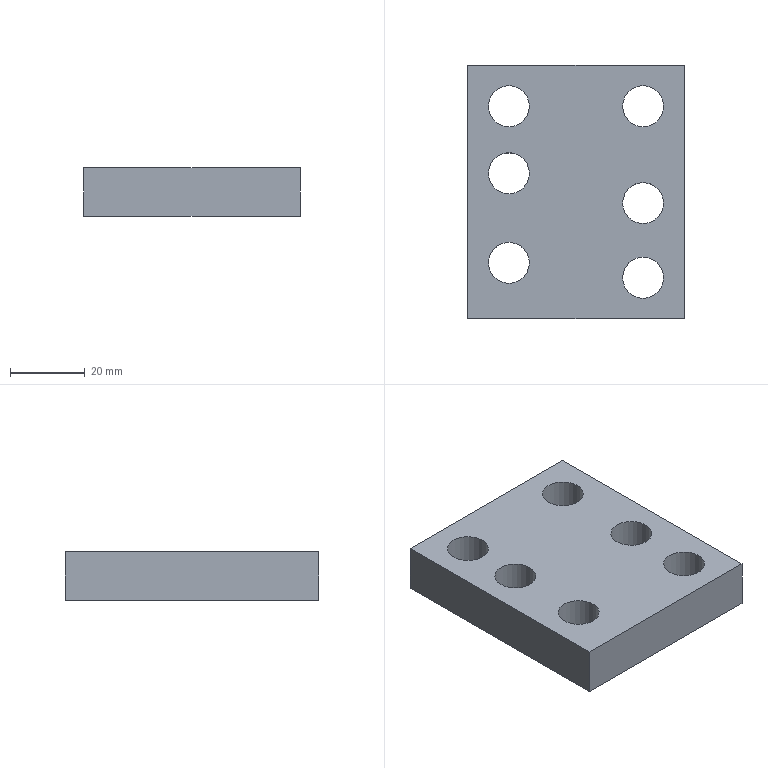Part | NX | features solid 2 | 1 solid | 12 faces | box 58 x 68 x 13 mm | volume 43859 mm3 | plane 6 | cylinder 6 | commonest cylinder face diameters 11 x6
STEP:
#1=CARTESIAN_POINT('',(1257.079,107.904,53.));
#2=VERTEX_POINT('',#1);
#3=CARTESIAN_POINT('',(1257.079,107.904,40.));
#4=VERTEX_POINT('',#3);
#5=CARTESIAN_POINT('',(1257.079,107.904,40.));
#6=DIRECTION('',(0.,0.,1.));
#7=VECTOR('',#6,1000.);
#8=LINE('',#5,#7);
#9=EDGE_CURVE('',#2,#4,#8,.F.);
#10=ORIENTED_EDGE('',*,*,#9,.T.);
#11=CARTESIAN_POINT('',(1315.079,107.904,40.));
#12=VERTEX_POINT('',#11);
#13=CARTESIAN_POINT('',(1286.079,107.904,40.));
#14=DIRECTION('',(1.,0.,0.));
#15=VECTOR('',#14,1000.);
#16=LINE('',#13,#15);
#17=EDGE_CURVE('',#12,#4,#16,.F.);
#18=ORIENTED_EDGE('',*,*,#17,.F.);
#19=CARTESIAN_POINT('',(1315.079,107.904,53.));
#20=VERTEX_POINT('',#19);
#21=CARTESIAN_POINT('',(1315.079,107.904,40.));
#22=DIRECTION('',(0.,0.,1.));
#23=VECTOR('',#22,1000.);
#24=LINE('',#21,#23);
#25=EDGE_CURVE('',#20,#12,#24,.F.);
#26=ORIENTED_EDGE('',*,*,#25,.F.);
#27=CARTESIAN_POINT('',(2087.158,107.904,53.));
#28=DIRECTION('',(1.,0.,0.));
#29=VECTOR('',#28,1000.);
#30=LINE('',#27,#29);
#31=EDGE_CURVE('',#20,#2,#30,.F.);
#32=ORIENTED_EDGE('',*,*,#31,.T.);
#33=EDGE_LOOP('',(#10,#18,#26,#32));
#34=FACE_BOUND('',#33,.T.);
#35=CARTESIAN_POINT('',(1286.079,107.904,40.));
#36=DIRECTION('',(0.,1.,0.));
#37=DIRECTION('',(1.,0.,0.));
#38=AXIS2_PLACEMENT_3D('',#35,#36,#37);
#39=PLANE('',#38);
#40=ADVANCED_FACE('',(#34),#39,.F.);
#41=ORIENTED_EDGE('',*,*,#25,.T.);
#42=CARTESIAN_POINT('',(1315.079,175.904,40.));
#43=VERTEX_POINT('',#42);
#44=CARTESIAN_POINT('',(1315.079,141.904,40.));
#45=DIRECTION('',(0.,1.,0.));
#46=VECTOR('',#45,1000.);
#47=LINE('',#44,#46);
#48=EDGE_CURVE('',#43,#12,#47,.F.);
#49=ORIENTED_EDGE('',*,*,#48,.F.);
#50=CARTESIAN_POINT('',(1315.079,175.904,53.));
#51=VERTEX_POINT('',#50);
#52=CARTESIAN_POINT('',(1315.079,175.904,40.));
#53=DIRECTION('',(0.,0.,1.));
#54=VECTOR('',#53,1000.);
#55=LINE('',#52,#54);
#56=EDGE_CURVE('',#51,#43,#55,.F.);
#57=ORIENTED_EDGE('',*,*,#56,.F.);
#58=CARTESIAN_POINT('',(1315.079,0.000000688,53.));
#59=DIRECTION('',(0.,1.,0.));
#60=VECTOR('',#59,1000.);
#61=LINE('',#58,#60);
#62=EDGE_CURVE('',#51,#20,#61,.F.);
#63=ORIENTED_EDGE('',*,*,#62,.T.);
#64=EDGE_LOOP('',(#41,#49,#57,#63));
#65=FACE_BOUND('',#64,.T.);
#66=CARTESIAN_POINT('',(1315.079,141.904,40.));
#67=DIRECTION('',(-1.,0.,0.));
#68=DIRECTION('',(0.,1.,0.));
#69=AXIS2_PLACEMENT_3D('',#66,#67,#68);
#70=PLANE('',#69);
#71=ADVANCED_FACE('',(#65),#70,.F.);
#72=ORIENTED_EDGE('',*,*,#56,.T.);
#73=CARTESIAN_POINT('',(1257.079,175.904,40.));
#74=VERTEX_POINT('',#73);
#75=CARTESIAN_POINT('',(1286.079,175.904,40.));
#76=DIRECTION('',(-1.,0.,0.));
#77=VECTOR('',#76,1000.);
#78=LINE('',#75,#77);
#79=EDGE_CURVE('',#74,#43,#78,.F.);
#80=ORIENTED_EDGE('',*,*,#79,.F.);
#81=CARTESIAN_POINT('',(1257.079,175.904,53.));
#82=VERTEX_POINT('',#81);
#83=CARTESIAN_POINT('',(1257.079,175.904,40.));
#84=DIRECTION('',(0.,0.,1.));
#85=VECTOR('',#84,1000.);
#86=LINE('',#83,#85);
#87=EDGE_CURVE('',#82,#74,#86,.F.);
#88=ORIENTED_EDGE('',*,*,#87,.F.);
#89=CARTESIAN_POINT('',(2087.158,175.904,53.));
#90=DIRECTION('',(-1.,0.,0.));
#91=VECTOR('',#90,1000.);
#92=LINE('',#89,#91);
#93=EDGE_CURVE('',#82,#51,#92,.F.);
#94=ORIENTED_EDGE('',*,*,#93,.T.);
#95=EDGE_LOOP('',(#72,#80,#88,#94));
#96=FACE_BOUND('',#95,.T.);
#97=CARTESIAN_POINT('',(1286.079,175.904,40.));
#98=DIRECTION('',(0.,-1.,0.));
#99=DIRECTION('',(-1.,0.,0.));
#100=AXIS2_PLACEMENT_3D('',#97,#98,#99);
#101=PLANE('',#100);
#102=ADVANCED_FACE('',(#96),#101,.F.);
#103=CARTESIAN_POINT('',(1273.579,146.904,40.));
#104=VERTEX_POINT('',#103);
#105=CARTESIAN_POINT('',(1268.079,146.904,40.));
#106=DIRECTION('',(0.,0.,-1.));
#107=DIRECTION('',(1.,0.,0.));
#108=AXIS2_PLACEMENT_3D('',#105,#106,#107);
#109=CIRCLE('',#108,5.5);
#110=EDGE_CURVE('',#104,#104,#109,.T.);
#111=ORIENTED_EDGE('',*,*,#110,.T.);
#112=EDGE_LOOP('',(#111));
#113=FACE_BOUND('',#112,.T.);
#114=CARTESIAN_POINT('',(1262.579,146.904,53.));
#115=VERTEX_POINT('',#114);
#116=CARTESIAN_POINT('',(1268.079,146.904,53.));
#117=DIRECTION('',(0.,0.,-1.));
#118=DIRECTION('',(-1.,0.,0.));
#119=AXIS2_PLACEMENT_3D('',#116,#117,#118);
#120=CIRCLE('',#119,5.5);
#121=EDGE_CURVE('',#115,#115,#120,.T.);
#122=ORIENTED_EDGE('',*,*,#121,.F.);
#123=EDGE_LOOP('',(#122));
#124=FACE_BOUND('',#123,.T.);
#125=CARTESIAN_POINT('',(1268.079,146.904,40.));
#126=DIRECTION('',(0.,0.,-1.));
#127=DIRECTION('',(1.,0.,0.));
#128=AXIS2_PLACEMENT_3D('',#125,#126,#127);
#129=CYLINDRICAL_SURFACE('',#128,5.5);
#130=ADVANCED_FACE('',(#113,#124),#129,.F.);
#131=CARTESIAN_POINT('',(1309.579,138.904,40.));
#132=VERTEX_POINT('',#131);
#133=CARTESIAN_POINT('',(1304.079,138.904,40.));
#134=DIRECTION('',(0.,0.,-1.));
#135=DIRECTION('',(1.,0.,0.));
#136=AXIS2_PLACEMENT_3D('',#133,#134,#135);
#137=CIRCLE('',#136,5.5);
#138=EDGE_CURVE('',#132,#132,#137,.F.);
#139=ORIENTED_EDGE('',*,*,#138,.F.);
#140=EDGE_LOOP('',(#139));
#141=FACE_BOUND('',#140,.T.);
#142=CARTESIAN_POINT('',(1298.579,138.904,53.));
#143=VERTEX_POINT('',#142);
#144=CARTESIAN_POINT('',(1304.079,138.904,53.));
#145=DIRECTION('',(0.,0.,-1.));
#146=DIRECTION('',(-1.,0.,0.));
#147=AXIS2_PLACEMENT_3D('',#144,#145,#146);
#148=CIRCLE('',#147,5.5);
#149=EDGE_CURVE('',#143,#143,#148,.F.);
#150=ORIENTED_EDGE('',*,*,#149,.T.);
#151=EDGE_LOOP('',(#150));
#152=FACE_BOUND('',#151,.T.);
#153=CARTESIAN_POINT('',(1304.079,138.904,40.));
#154=DIRECTION('',(0.,0.,-1.));
#155=DIRECTION('',(1.,0.,0.));
#156=AXIS2_PLACEMENT_3D('',#153,#154,#155);
#157=CYLINDRICAL_SURFACE('',#156,5.5);
#158=ADVANCED_FACE('',(#141,#152),#157,.F.);
#159=CARTESIAN_POINT('',(1273.579,122.904,40.));
#160=VERTEX_POINT('',#159);
#161=CARTESIAN_POINT('',(1268.079,122.904,40.));
#162=DIRECTION('',(0.,0.,-1.));
#163=DIRECTION('',(1.,0.,0.));
#164=AXIS2_PLACEMENT_3D('',#161,#162,#163);
#165=CIRCLE('',#164,5.5);
#166=EDGE_CURVE('',#160,#160,#165,.T.);
#167=ORIENTED_EDGE('',*,*,#166,.T.);
#168=EDGE_LOOP('',(#167));
#169=FACE_BOUND('',#168,.T.);
#170=CARTESIAN_POINT('',(1262.579,122.904,53.));
#171=VERTEX_POINT('',#170);
#172=CARTESIAN_POINT('',(1268.079,122.904,53.));
#173=DIRECTION('',(0.,0.,-1.));
#174=DIRECTION('',(-1.,0.,0.));
#175=AXIS2_PLACEMENT_3D('',#172,#173,#174);
#176=CIRCLE('',#175,5.5);
#177=EDGE_CURVE('',#171,#171,#176,.T.);
#178=ORIENTED_EDGE('',*,*,#177,.F.);
#179=EDGE_LOOP('',(#178));
#180=FACE_BOUND('',#179,.T.);
#181=CARTESIAN_POINT('',(1268.079,122.904,40.));
#182=DIRECTION('',(0.,0.,-1.));
#183=DIRECTION('',(1.,0.,0.));
#184=AXIS2_PLACEMENT_3D('',#181,#182,#183);
#185=CYLINDRICAL_SURFACE('',#184,5.5);
#186=ADVANCED_FACE('',(#169,#180),#185,.F.);
#187=CARTESIAN_POINT('',(1273.579,164.904,40.));
#188=VERTEX_POINT('',#187);
#189=CARTESIAN_POINT('',(1268.079,164.904,40.));
#190=DIRECTION('',(0.,0.,-1.));
#191=DIRECTION('',(1.,0.,0.));
#192=AXIS2_PLACEMENT_3D('',#189,#190,#191);
#193=CIRCLE('',#192,5.5);
#194=EDGE_CURVE('',#188,#188,#193,.T.);
#195=ORIENTED_EDGE('',*,*,#194,.T.);
#196=EDGE_LOOP('',(#195));
#197=FACE_BOUND('',#196,.T.);
#198=CARTESIAN_POINT('',(1262.579,164.904,53.));
#199=VERTEX_POINT('',#198);
#200=CARTESIAN_POINT('',(1268.079,164.904,53.));
#201=DIRECTION('',(0.,0.,-1.));
#202=DIRECTION('',(-1.,0.,0.));
#203=AXIS2_PLACEMENT_3D('',#200,#201,#202);
#204=CIRCLE('',#203,5.5);
#205=EDGE_CURVE('',#199,#199,#204,.T.);
#206=ORIENTED_EDGE('',*,*,#205,.F.);
#207=EDGE_LOOP('',(#206));
#208=FACE_BOUND('',#207,.T.);
#209=CARTESIAN_POINT('',(1268.079,164.904,40.));
#210=DIRECTION('',(0.,0.,-1.));
#211=DIRECTION('',(1.,0.,0.));
#212=AXIS2_PLACEMENT_3D('',#209,#210,#211);
#213=CYLINDRICAL_SURFACE('',#212,5.5);
#214=ADVANCED_FACE('',(#197,#208),#213,.F.);
#215=CARTESIAN_POINT('',(1309.579,164.904,40.));
#216=VERTEX_POINT('',#215);
#217=CARTESIAN_POINT('',(1304.079,164.904,40.));
#218=DIRECTION('',(0.,0.,-1.));
#219=DIRECTION('',(1.,0.,0.));
#220=AXIS2_PLACEMENT_3D('',#217,#218,#219);
#221=CIRCLE('',#220,5.5);
#222=EDGE_CURVE('',#216,#216,#221,.T.);
#223=ORIENTED_EDGE('',*,*,#222,.T.);
#224=EDGE_LOOP('',(#223));
#225=FACE_BOUND('',#224,.T.);
#226=CARTESIAN_POINT('',(1298.579,164.904,53.));
#227=VERTEX_POINT('',#226);
#228=CARTESIAN_POINT('',(1304.079,164.904,53.));
#229=DIRECTION('',(0.,0.,-1.));
#230=DIRECTION('',(-1.,0.,0.));
#231=AXIS2_PLACEMENT_3D('',#228,#229,#230);
#232=CIRCLE('',#231,5.5);
#233=EDGE_CURVE('',#227,#227,#232,.T.);
#234=ORIENTED_EDGE('',*,*,#233,.F.);
#235=EDGE_LOOP('',(#234));
#236=FACE_BOUND('',#235,.T.);
#237=CARTESIAN_POINT('',(1304.079,164.904,40.));
#238=DIRECTION('',(0.,0.,-1.));
#239=DIRECTION('',(1.,0.,0.));
#240=AXIS2_PLACEMENT_3D('',#237,#238,#239);
#241=CYLINDRICAL_SURFACE('',#240,5.5);
#242=ADVANCED_FACE('',(#225,#236),#241,.F.);
#243=CARTESIAN_POINT('',(1309.579,118.904,40.));
#244=VERTEX_POINT('',#243);
#245=CARTESIAN_POINT('',(1304.079,118.904,40.));
#246=DIRECTION('',(0.,0.,-1.));
#247=DIRECTION('',(1.,0.,0.));
#248=AXIS2_PLACEMENT_3D('',#245,#246,#247);
#249=CIRCLE('',#248,5.5);
#250=EDGE_CURVE('',#244,#244,#249,.F.);
#251=ORIENTED_EDGE('',*,*,#250,.F.);
#252=EDGE_LOOP('',(#251));
#253=FACE_BOUND('',#252,.T.);
#254=CARTESIAN_POINT('',(1298.579,118.904,53.));
#255=VERTEX_POINT('',#254);
#256=CARTESIAN_POINT('',(1304.079,118.904,53.));
#257=DIRECTION('',(0.,0.,-1.));
#258=DIRECTION('',(-1.,0.,0.));
#259=AXIS2_PLACEMENT_3D('',#256,#257,#258);
#260=CIRCLE('',#259,5.5);
#261=EDGE_CURVE('',#255,#255,#260,.F.);
#262=ORIENTED_EDGE('',*,*,#261,.T.);
#263=EDGE_LOOP('',(#262));
#264=FACE_BOUND('',#263,.T.);
#265=CARTESIAN_POINT('',(1304.079,118.904,40.));
#266=DIRECTION('',(0.,0.,-1.));
#267=DIRECTION('',(1.,0.,0.));
#268=AXIS2_PLACEMENT_3D('',#265,#266,#267);
#269=CYLINDRICAL_SURFACE('',#268,5.5);
#270=ADVANCED_FACE('',(#253,#264),#269,.F.);
#271=CARTESIAN_POINT('',(1257.079,0.000000688,53.));
#272=DIRECTION('',(0.,-1.,0.));
#273=VECTOR('',#272,1000.);
#274=LINE('',#271,#273);
#275=EDGE_CURVE('',#2,#82,#274,.F.);
#276=ORIENTED_EDGE('',*,*,#275,.T.);
#277=ORIENTED_EDGE('',*,*,#87,.T.);
#278=CARTESIAN_POINT('',(1257.079,141.904,40.));
#279=DIRECTION('',(0.,-1.,0.));
#280=VECTOR('',#279,1000.);
#281=LINE('',#278,#280);
#282=EDGE_CURVE('',#4,#74,#281,.F.);
#283=ORIENTED_EDGE('',*,*,#282,.F.);
#284=ORIENTED_EDGE('',*,*,#9,.F.);
#285=EDGE_LOOP('',(#276,#277,#283,#284));
#286=FACE_BOUND('',#285,.T.);
#287=CARTESIAN_POINT('',(1257.079,141.904,40.));
#288=DIRECTION('',(1.,0.,0.));
#289=DIRECTION('',(0.,-1.,0.));
#290=AXIS2_PLACEMENT_3D('',#287,#288,#289);
#291=PLANE('',#290);
#292=ADVANCED_FACE('',(#286),#291,.F.);
#293=ORIENTED_EDGE('',*,*,#110,.F.);
#294=EDGE_LOOP('',(#293));
#295=FACE_BOUND('',#294,.T.);
#296=ORIENTED_EDGE('',*,*,#138,.T.);
#297=EDGE_LOOP('',(#296));
#298=FACE_BOUND('',#297,.T.);
#299=ORIENTED_EDGE('',*,*,#166,.F.);
#300=EDGE_LOOP('',(#299));
#301=FACE_BOUND('',#300,.T.);
#302=ORIENTED_EDGE('',*,*,#194,.F.);
#303=EDGE_LOOP('',(#302));
#304=FACE_BOUND('',#303,.T.);
#305=ORIENTED_EDGE('',*,*,#222,.F.);
#306=EDGE_LOOP('',(#305));
#307=FACE_BOUND('',#306,.T.);
#308=ORIENTED_EDGE('',*,*,#250,.T.);
#309=EDGE_LOOP('',(#308));
#310=FACE_BOUND('',#309,.T.);
#311=ORIENTED_EDGE('',*,*,#79,.T.);
#312=ORIENTED_EDGE('',*,*,#48,.T.);
#313=ORIENTED_EDGE('',*,*,#17,.T.);
#314=ORIENTED_EDGE('',*,*,#282,.T.);
#315=EDGE_LOOP('',(#311,#312,#313,#314));
#316=FACE_BOUND('',#315,.T.);
#317=CARTESIAN_POINT('',(2087.158,0.000000688,40.));
#318=DIRECTION('',(0.,0.,-1.));
#319=DIRECTION('',(1.,0.,0.));
#320=AXIS2_PLACEMENT_3D('',#317,#318,#319);
#321=PLANE('',#320);
#322=ADVANCED_FACE('',(#295,#298,#301,#304,#307,#310,#316),#321,.T.);
#323=ORIENTED_EDGE('',*,*,#121,.T.);
#324=EDGE_LOOP('',(#323));
#325=FACE_BOUND('',#324,.T.);
#326=ORIENTED_EDGE('',*,*,#149,.F.);
#327=EDGE_LOOP('',(#326));
#328=FACE_BOUND('',#327,.T.);
#329=ORIENTED_EDGE('',*,*,#177,.T.);
#330=EDGE_LOOP('',(#329));
#331=FACE_BOUND('',#330,.T.);
#332=ORIENTED_EDGE('',*,*,#205,.T.);
#333=EDGE_LOOP('',(#332));
#334=FACE_BOUND('',#333,.T.);
#335=ORIENTED_EDGE('',*,*,#233,.T.);
#336=EDGE_LOOP('',(#335));
#337=FACE_BOUND('',#336,.T.);
#338=ORIENTED_EDGE('',*,*,#261,.F.);
#339=EDGE_LOOP('',(#338));
#340=FACE_BOUND('',#339,.T.);
#341=ORIENTED_EDGE('',*,*,#93,.F.);
#342=ORIENTED_EDGE('',*,*,#275,.F.);
#343=ORIENTED_EDGE('',*,*,#31,.F.);
#344=ORIENTED_EDGE('',*,*,#62,.F.);
#345=EDGE_LOOP('',(#341,#342,#343,#344));
#346=FACE_BOUND('',#345,.T.);
#347=CARTESIAN_POINT('',(2087.158,0.000000688,53.));
#348=DIRECTION('',(0.,0.,-1.));
#349=DIRECTION('',(1.,0.,0.));
#350=AXIS2_PLACEMENT_3D('',#347,#348,#349);
#351=PLANE('',#350);
#352=ADVANCED_FACE('',(#325,#328,#331,#334,#337,#340,#346),#351,.F.);
#353=CLOSED_SHELL('',(#40,#71,#102,#130,#158,#186,#214,#242,#270,#292,#322,#352));
#354=MANIFOLD_SOLID_BREP('',#353);
#355=(LENGTH_UNIT()NAMED_UNIT(*)SI_UNIT(.MILLI.,.METRE.));
#356=UNCERTAINTY_MEASURE_WITH_UNIT(LENGTH_MEASURE(0.00001),#355,'','');
#357=(NAMED_UNIT(*)PLANE_ANGLE_UNIT()SI_UNIT($,.RADIAN.));
#358=(NAMED_UNIT(*)SI_UNIT($,.STERADIAN.)SOLID_ANGLE_UNIT());
#359=(GEOMETRIC_REPRESENTATION_CONTEXT(3)GLOBAL_UNCERTAINTY_ASSIGNED_CONTEXT((#356))GLOBAL_UNIT_ASSIGNED_CONTEXT((#355,#357,#358))REPRESENTATION_CONTEXT('',''));
#360=ADVANCED_BREP_SHAPE_REPRESENTATION('',(#354),#359);